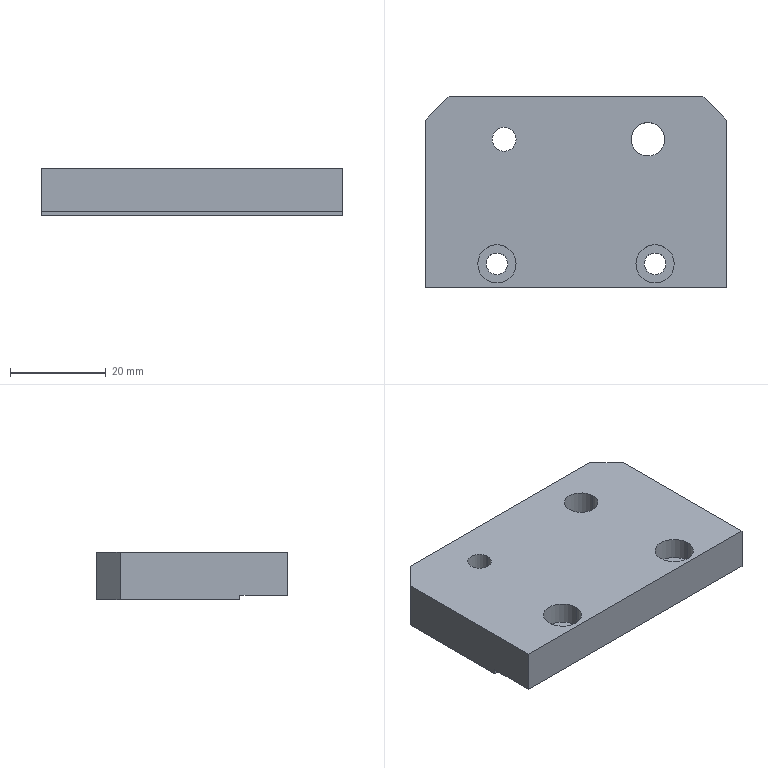Part | STEP file | 2034 Buffer mounting plate | 1 solid | 24 faces | box 63 x 40 x 10 mm | volume 23136 mm3 | cylinder 12 | plane 12 | commonest cylinder face diameters 4.5 x4 8 x4 5 x2 7 x2